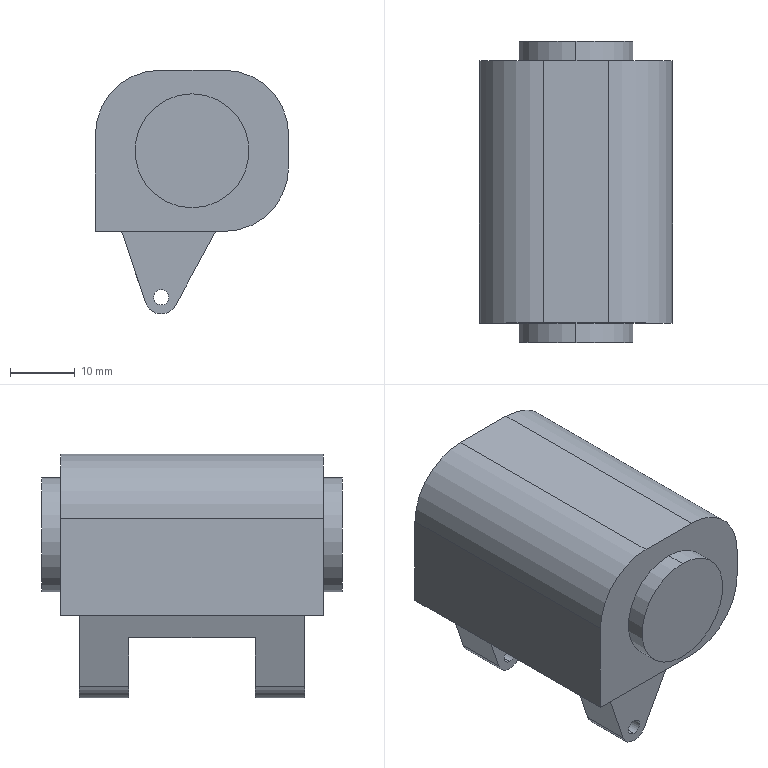Part | SolidWorks | features ICE 3, Cut 1, Extrusion 1, Fillet 1 | 1 solid | 28 faces | box 29.956 x 46.658 x 37.777 mm | volume 31870 mm3 | plane 15 | cylinder 13 | commonest cylinder face diameters 2.359 x4 17.683 x4 20 x3 5.115 x2
STEP:
#1=CARTESIAN_POINT('',(-25.009,23.329,21.342));
#2=VERTEX_POINT('',#1);
#3=CARTESIAN_POINT('',(-25.009,23.329,3.658));
#4=VERTEX_POINT('',#3);
#5=CARTESIAN_POINT('',(-25.009,23.329,12.5));
#6=DIRECTION('',(0.,1.,0.));
#7=DIRECTION('',(0.,0.,1.));
#8=AXIS2_PLACEMENT_3D('',#5,#6,#7);
#9=CIRCLE('',#8,8.842);
#10=EDGE_CURVE('',#2,#4,#9,.T.);
#11=ORIENTED_EDGE('',*,*,#10,.F.);
#12=CARTESIAN_POINT('',(-25.009,20.329,21.342));
#13=VERTEX_POINT('',#12);
#14=CARTESIAN_POINT('',(-25.009,23.329,21.342));
#15=DIRECTION('',(0.,-1.,0.));
#16=VECTOR('',#15,1000.);
#17=LINE('',#14,#16);
#18=EDGE_CURVE('',#2,#13,#17,.T.);
#19=ORIENTED_EDGE('',*,*,#18,.T.);
#20=CARTESIAN_POINT('',(-25.009,20.329,3.658));
#21=VERTEX_POINT('',#20);
#22=CARTESIAN_POINT('',(-25.009,20.329,12.5));
#23=DIRECTION('',(0.,1.,0.));
#24=DIRECTION('',(0.,0.,1.));
#25=AXIS2_PLACEMENT_3D('',#22,#23,#24);
#26=CIRCLE('',#25,8.842);
#27=EDGE_CURVE('',#13,#21,#26,.T.);
#28=ORIENTED_EDGE('',*,*,#27,.T.);
#29=CARTESIAN_POINT('',(-25.009,23.329,3.658));
#30=DIRECTION('',(0.,-1.,0.));
#31=VECTOR('',#30,1000.);
#32=LINE('',#29,#31);
#33=EDGE_CURVE('',#4,#21,#32,.T.);
#34=ORIENTED_EDGE('',*,*,#33,.F.);
#35=EDGE_LOOP('',(#11,#19,#28,#34));
#36=FACE_OUTER_BOUND('',#35,.T.);
#37=CARTESIAN_POINT('',(-25.009,23.329,12.5));
#38=DIRECTION('',(0.,-1.,0.));
#39=DIRECTION('',(0.,0.,-1.));
#40=AXIS2_PLACEMENT_3D('',#37,#38,#39);
#41=CYLINDRICAL_SURFACE('',#40,8.842);
#42=ADVANCED_FACE('',(#36),#41,.T.);
#43=CARTESIAN_POINT('',(-25.009,-23.329,3.658));
#44=VERTEX_POINT('',#43);
#45=CARTESIAN_POINT('',(-25.009,-23.329,21.342));
#46=VERTEX_POINT('',#45);
#47=CARTESIAN_POINT('',(-25.009,-23.329,12.5));
#48=DIRECTION('',(0.,-1.,0.));
#49=DIRECTION('',(0.,0.,-1.));
#50=AXIS2_PLACEMENT_3D('',#47,#48,#49);
#51=CIRCLE('',#50,8.842);
#52=EDGE_CURVE('',#44,#46,#51,.T.);
#53=ORIENTED_EDGE('',*,*,#52,.F.);
#54=CARTESIAN_POINT('',(-25.009,-20.329,3.658));
#55=VERTEX_POINT('',#54);
#56=CARTESIAN_POINT('',(-25.009,-23.329,3.658));
#57=DIRECTION('',(0.,1.,0.));
#58=VECTOR('',#57,1000.);
#59=LINE('',#56,#58);
#60=EDGE_CURVE('',#44,#55,#59,.T.);
#61=ORIENTED_EDGE('',*,*,#60,.T.);
#62=CARTESIAN_POINT('',(-25.009,-20.329,21.342));
#63=VERTEX_POINT('',#62);
#64=CARTESIAN_POINT('',(-25.009,-20.329,12.5));
#65=DIRECTION('',(0.,-1.,0.));
#66=DIRECTION('',(0.,0.,-1.));
#67=AXIS2_PLACEMENT_3D('',#64,#65,#66);
#68=CIRCLE('',#67,8.842);
#69=EDGE_CURVE('',#55,#63,#68,.T.);
#70=ORIENTED_EDGE('',*,*,#69,.T.);
#71=CARTESIAN_POINT('',(-25.009,-23.329,21.342));
#72=DIRECTION('',(0.,1.,0.));
#73=VECTOR('',#72,1000.);
#74=LINE('',#71,#73);
#75=EDGE_CURVE('',#46,#63,#74,.T.);
#76=ORIENTED_EDGE('',*,*,#75,.F.);
#77=EDGE_LOOP('',(#53,#61,#70,#76));
#78=FACE_OUTER_BOUND('',#77,.T.);
#79=CARTESIAN_POINT('',(-25.009,-23.329,12.5));
#80=DIRECTION('',(0.,1.,0.));
#81=DIRECTION('',(0.,0.,1.));
#82=AXIS2_PLACEMENT_3D('',#79,#80,#81);
#83=CYLINDRICAL_SURFACE('',#82,8.842);
#84=ADVANCED_FACE('',(#78),#83,.T.);
#85=CARTESIAN_POINT('',(-29.791,-17.5,-9.04));
#86=VERTEX_POINT('',#85);
#87=CARTESIAN_POINT('',(-29.791,-17.5,-11.399));
#88=VERTEX_POINT('',#87);
#89=CARTESIAN_POINT('',(-29.791,-17.5,-10.22));
#90=DIRECTION('',(0.,-1.,0.));
#91=DIRECTION('',(0.,0.,-1.));
#92=AXIS2_PLACEMENT_3D('',#89,#90,#91);
#93=CIRCLE('',#92,1.179);
#94=EDGE_CURVE('',#86,#88,#93,.T.);
#95=ORIENTED_EDGE('',*,*,#94,.T.);
#96=CARTESIAN_POINT('',(-29.791,-9.777,-11.399));
#97=VERTEX_POINT('',#96);
#98=CARTESIAN_POINT('',(-29.791,-17.5,-11.399));
#99=DIRECTION('',(0.,1.,0.));
#100=VECTOR('',#99,1000.);
#101=LINE('',#98,#100);
#102=EDGE_CURVE('',#88,#97,#101,.T.);
#103=ORIENTED_EDGE('',*,*,#102,.T.);
#104=CARTESIAN_POINT('',(-29.791,-9.777,-9.04));
#105=VERTEX_POINT('',#104);
#106=CARTESIAN_POINT('',(-29.791,-9.777,-10.22));
#107=DIRECTION('',(0.,-1.,0.));
#108=DIRECTION('',(0.,0.,-1.));
#109=AXIS2_PLACEMENT_3D('',#106,#107,#108);
#110=CIRCLE('',#109,1.179);
#111=EDGE_CURVE('',#105,#97,#110,.T.);
#112=ORIENTED_EDGE('',*,*,#111,.F.);
#113=CARTESIAN_POINT('',(-29.791,-17.5,-9.04));
#114=DIRECTION('',(0.,1.,0.));
#115=VECTOR('',#114,1000.);
#116=LINE('',#113,#115);
#117=EDGE_CURVE('',#86,#105,#116,.T.);
#118=ORIENTED_EDGE('',*,*,#117,.F.);
#119=EDGE_LOOP('',(#95,#103,#112,#118));
#120=FACE_OUTER_BOUND('',#119,.T.);
#121=CARTESIAN_POINT('',(-29.791,-17.5,-10.22));
#122=DIRECTION('',(0.,1.,0.));
#123=DIRECTION('',(0.,0.,1.));
#124=AXIS2_PLACEMENT_3D('',#121,#122,#123);
#125=CYLINDRICAL_SURFACE('',#124,1.179);
#126=ADVANCED_FACE('',(#120),#125,.F.);
#127=CARTESIAN_POINT('',(-29.791,9.777,-11.399));
#128=VERTEX_POINT('',#127);
#129=CARTESIAN_POINT('',(-29.791,9.777,-9.04));
#130=VERTEX_POINT('',#129);
#131=CARTESIAN_POINT('',(-29.791,9.777,-10.22));
#132=DIRECTION('',(0.,1.,0.));
#133=DIRECTION('',(0.,0.,1.));
#134=AXIS2_PLACEMENT_3D('',#131,#132,#133);
#135=CIRCLE('',#134,1.179);
#136=EDGE_CURVE('',#128,#130,#135,.T.);
#137=ORIENTED_EDGE('',*,*,#136,.F.);
#138=CARTESIAN_POINT('',(-29.791,17.5,-11.399));
#139=VERTEX_POINT('',#138);
#140=CARTESIAN_POINT('',(-29.791,-17.5,-11.399));
#141=DIRECTION('',(0.,1.,0.));
#142=VECTOR('',#141,1000.);
#143=LINE('',#140,#142);
#144=EDGE_CURVE('',#128,#139,#143,.T.);
#145=ORIENTED_EDGE('',*,*,#144,.T.);
#146=CARTESIAN_POINT('',(-29.791,17.5,-9.04));
#147=VERTEX_POINT('',#146);
#148=CARTESIAN_POINT('',(-29.791,17.5,-10.22));
#149=DIRECTION('',(0.,-1.,0.));
#150=DIRECTION('',(0.,0.,-1.));
#151=AXIS2_PLACEMENT_3D('',#148,#149,#150);
#152=CIRCLE('',#151,1.179);
#153=EDGE_CURVE('',#147,#139,#152,.T.);
#154=ORIENTED_EDGE('',*,*,#153,.F.);
#155=CARTESIAN_POINT('',(-29.791,-17.5,-9.04));
#156=DIRECTION('',(0.,1.,0.));
#157=VECTOR('',#156,1000.);
#158=LINE('',#155,#157);
#159=EDGE_CURVE('',#130,#147,#158,.T.);
#160=ORIENTED_EDGE('',*,*,#159,.F.);
#161=EDGE_LOOP('',(#137,#145,#154,#160));
#162=FACE_OUTER_BOUND('',#161,.T.);
#163=CARTESIAN_POINT('',(-29.791,-17.5,-10.22));
#164=DIRECTION('',(0.,1.,0.));
#165=DIRECTION('',(0.,0.,1.));
#166=AXIS2_PLACEMENT_3D('',#163,#164,#165);
#167=CYLINDRICAL_SURFACE('',#166,1.179);
#168=ADVANCED_FACE('',(#162),#167,.F.);
#169=CARTESIAN_POINT('',(-27.542,9.777,-11.438));
#170=VERTEX_POINT('',#169);
#171=CARTESIAN_POINT('',(-27.542,17.5,-11.438));
#172=VERTEX_POINT('',#171);
#173=CARTESIAN_POINT('',(-27.542,-17.5,-11.438));
#174=DIRECTION('',(0.,1.,0.));
#175=VECTOR('',#174,1000.);
#176=LINE('',#173,#175);
#177=EDGE_CURVE('',#170,#172,#176,.T.);
#178=ORIENTED_EDGE('',*,*,#177,.F.);
#179=CARTESIAN_POINT('',(-32.216,9.777,-11.033));
#180=VERTEX_POINT('',#179);
#181=CARTESIAN_POINT('',(-29.791,9.777,-10.22));
#182=DIRECTION('',(0.,1.,0.));
#183=DIRECTION('',(0.,0.,1.));
#184=AXIS2_PLACEMENT_3D('',#181,#182,#183);
#185=CIRCLE('',#184,2.558);
#186=EDGE_CURVE('',#170,#180,#185,.T.);
#187=ORIENTED_EDGE('',*,*,#186,.T.);
#188=CARTESIAN_POINT('',(-32.216,17.5,-11.033));
#189=VERTEX_POINT('',#188);
#190=CARTESIAN_POINT('',(-32.216,-17.5,-11.033));
#191=DIRECTION('',(0.,1.,0.));
#192=VECTOR('',#191,1000.);
#193=LINE('',#190,#192);
#194=EDGE_CURVE('',#180,#189,#193,.T.);
#195=ORIENTED_EDGE('',*,*,#194,.T.);
#196=CARTESIAN_POINT('',(-29.791,17.5,-10.22));
#197=DIRECTION('',(0.,-1.,0.));
#198=DIRECTION('',(0.,0.,-1.));
#199=AXIS2_PLACEMENT_3D('',#196,#197,#198);
#200=CIRCLE('',#199,2.558);
#201=EDGE_CURVE('',#189,#172,#200,.T.);
#202=ORIENTED_EDGE('',*,*,#201,.T.);
#203=EDGE_LOOP('',(#178,#187,#195,#202));
#204=FACE_OUTER_BOUND('',#203,.T.);
#205=CARTESIAN_POINT('',(-29.791,-17.5,-10.22));
#206=DIRECTION('',(0.,1.,0.));
#207=DIRECTION('',(0.,0.,1.));
#208=AXIS2_PLACEMENT_3D('',#205,#206,#207);
#209=CYLINDRICAL_SURFACE('',#208,2.558);
#210=ADVANCED_FACE('',(#204),#209,.T.);
#211=ORIENTED_EDGE('',*,*,#144,.F.);
#212=CARTESIAN_POINT('',(-29.791,9.777,-10.22));
#213=DIRECTION('',(0.,1.,0.));
#214=DIRECTION('',(0.,0.,1.));
#215=AXIS2_PLACEMENT_3D('',#212,#213,#214);
#216=CIRCLE('',#215,1.179);
#217=EDGE_CURVE('',#130,#128,#216,.T.);
#218=ORIENTED_EDGE('',*,*,#217,.F.);
#219=ORIENTED_EDGE('',*,*,#159,.T.);
#220=CARTESIAN_POINT('',(-29.791,17.5,-10.22));
#221=DIRECTION('',(0.,-1.,0.));
#222=DIRECTION('',(0.,0.,-1.));
#223=AXIS2_PLACEMENT_3D('',#220,#221,#222);
#224=CIRCLE('',#223,1.179);
#225=EDGE_CURVE('',#139,#147,#224,.T.);
#226=ORIENTED_EDGE('',*,*,#225,.F.);
#227=EDGE_LOOP('',(#211,#218,#219,#226));
#228=FACE_OUTER_BOUND('',#227,.T.);
#229=CARTESIAN_POINT('',(-29.791,-17.5,-10.22));
#230=DIRECTION('',(0.,1.,0.));
#231=DIRECTION('',(0.,0.,1.));
#232=AXIS2_PLACEMENT_3D('',#229,#230,#231);
#233=CYLINDRICAL_SURFACE('',#232,1.179);
#234=ADVANCED_FACE('',(#228),#233,.F.);
#235=CARTESIAN_POINT('',(-10.031,-20.329,15.));
#236=VERTEX_POINT('',#235);
#237=CARTESIAN_POINT('',(-10.031,-20.329,10.));
#238=VERTEX_POINT('',#237);
#239=CARTESIAN_POINT('',(-10.031,-20.329,25.));
#240=DIRECTION('',(0.,0.,-1.));
#241=VECTOR('',#240,1000.);
#242=LINE('',#239,#241);
#243=EDGE_CURVE('',#236,#238,#242,.T.);
#244=ORIENTED_EDGE('',*,*,#243,.T.);
#245=CARTESIAN_POINT('',(-10.031,20.329,10.));
#246=VERTEX_POINT('',#245);
#247=CARTESIAN_POINT('',(-10.031,20.329,10.));
#248=DIRECTION('',(0.,1.,0.));
#249=VECTOR('',#248,1000.);
#250=LINE('',#247,#249);
#251=EDGE_CURVE('',#238,#246,#250,.T.);
#252=ORIENTED_EDGE('',*,*,#251,.T.);
#253=CARTESIAN_POINT('',(-10.031,20.329,15.));
#254=VERTEX_POINT('',#253);
#255=CARTESIAN_POINT('',(-10.031,20.329,25.));
#256=DIRECTION('',(0.,0.,-1.));
#257=VECTOR('',#256,1000.);
#258=LINE('',#255,#257);
#259=EDGE_CURVE('',#254,#246,#258,.T.);
#260=ORIENTED_EDGE('',*,*,#259,.F.);
#261=CARTESIAN_POINT('',(-10.031,-20.329,15.));
#262=DIRECTION('',(0.,-1.,0.));
#263=VECTOR('',#262,1000.);
#264=LINE('',#261,#263);
#265=EDGE_CURVE('',#254,#236,#264,.T.);
#266=ORIENTED_EDGE('',*,*,#265,.T.);
#267=EDGE_LOOP('',(#244,#252,#260,#266));
#268=FACE_OUTER_BOUND('',#267,.T.);
#269=CARTESIAN_POINT('',(-10.031,20.329,25.));
#270=DIRECTION('',(-1.,0.,0.));
#271=DIRECTION('',(0.,0.,1.));
#272=AXIS2_PLACEMENT_3D('',#269,#270,#271);
#273=PLANE('',#272);
#274=ADVANCED_FACE('',(#268),#273,.F.);
#275=CARTESIAN_POINT('',(-25.009,20.329,12.5));
#276=DIRECTION('',(0.,1.,0.));
#277=DIRECTION('',(0.,0.,1.));
#278=AXIS2_PLACEMENT_3D('',#275,#276,#277);
#279=CIRCLE('',#278,8.842);
#280=EDGE_CURVE('',#21,#13,#279,.T.);
#281=ORIENTED_EDGE('',*,*,#280,.F.);
#282=ORIENTED_EDGE('',*,*,#27,.F.);
#283=EDGE_LOOP('',(#281,#282));
#284=FACE_BOUND('',#283,.T.);
#285=CARTESIAN_POINT('',(-39.987,20.329,15.));
#286=VERTEX_POINT('',#285);
#287=CARTESIAN_POINT('',(-39.987,20.329,0.));
#288=VERTEX_POINT('',#287);
#289=CARTESIAN_POINT('',(-39.987,20.329,25.));
#290=DIRECTION('',(0.,0.,-1.));
#291=VECTOR('',#290,1000.);
#292=LINE('',#289,#291);
#293=EDGE_CURVE('',#286,#288,#292,.T.);
#294=ORIENTED_EDGE('',*,*,#293,.F.);
#295=CARTESIAN_POINT('',(-29.987,20.329,25.));
#296=VERTEX_POINT('',#295);
#297=CARTESIAN_POINT('',(-29.987,20.329,15.));
#298=DIRECTION('',(0.,1.,0.));
#299=DIRECTION('',(0.,0.,-1.));
#300=AXIS2_PLACEMENT_3D('',#297,#298,#299);
#301=CIRCLE('',#300,10.);
#302=EDGE_CURVE('',#286,#296,#301,.T.);
#303=ORIENTED_EDGE('',*,*,#302,.T.);
#304=CARTESIAN_POINT('',(-20.031,20.329,25.));
#305=VERTEX_POINT('',#304);
#306=CARTESIAN_POINT('',(-39.987,20.329,25.));
#307=DIRECTION('',(-1.,0.,0.));
#308=VECTOR('',#307,1000.);
#309=LINE('',#306,#308);
#310=EDGE_CURVE('',#305,#296,#309,.T.);
#311=ORIENTED_EDGE('',*,*,#310,.F.);
#312=CARTESIAN_POINT('',(-20.031,20.329,15.));
#313=DIRECTION('',(0.,1.,0.));
#314=DIRECTION('',(0.,0.,-1.));
#315=AXIS2_PLACEMENT_3D('',#312,#313,#314);
#316=CIRCLE('',#315,10.);
#317=EDGE_CURVE('',#305,#254,#316,.T.);
#318=ORIENTED_EDGE('',*,*,#317,.T.);
#319=ORIENTED_EDGE('',*,*,#259,.T.);
#320=CARTESIAN_POINT('',(-20.031,20.329,0.));
#321=VERTEX_POINT('',#320);
#322=CARTESIAN_POINT('',(-20.031,20.329,10.));
#323=DIRECTION('',(0.,1.,0.));
#324=DIRECTION('',(0.,0.,-1.));
#325=AXIS2_PLACEMENT_3D('',#322,#323,#324);
#326=CIRCLE('',#325,10.);
#327=EDGE_CURVE('',#246,#321,#326,.T.);
#328=ORIENTED_EDGE('',*,*,#327,.T.);
#329=CARTESIAN_POINT('',(-39.987,20.329,0.));
#330=DIRECTION('',(-1.,0.,0.));
#331=VECTOR('',#330,1000.);
#332=LINE('',#329,#331);
#333=EDGE_CURVE('',#321,#288,#332,.T.);
#334=ORIENTED_EDGE('',*,*,#333,.T.);
#335=EDGE_LOOP('',(#294,#303,#311,#318,#319,#328,#334));
#336=FACE_OUTER_BOUND('',#335,.T.);
#337=CARTESIAN_POINT('',(-39.987,20.329,25.));
#338=DIRECTION('',(0.,-1.,0.));
#339=DIRECTION('',(0.,0.,-1.));
#340=AXIS2_PLACEMENT_3D('',#337,#338,#339);
#341=PLANE('',#340);
#342=ADVANCED_FACE('',(#284,#336),#341,.F.);
#343=CARTESIAN_POINT('',(-39.987,-20.329,15.));
#344=VERTEX_POINT('',#343);
#345=CARTESIAN_POINT('',(-39.987,-20.329,0.));
#346=VERTEX_POINT('',#345);
#347=CARTESIAN_POINT('',(-39.987,-20.329,25.));
#348=DIRECTION('',(0.,0.,-1.));
#349=VECTOR('',#348,1000.);
#350=LINE('',#347,#349);
#351=EDGE_CURVE('',#344,#346,#350,.T.);
#352=ORIENTED_EDGE('',*,*,#351,.F.);
#353=CARTESIAN_POINT('',(-39.987,20.329,15.));
#354=DIRECTION('',(0.,1.,0.));
#355=VECTOR('',#354,1000.);
#356=LINE('',#353,#355);
#357=EDGE_CURVE('',#344,#286,#356,.T.);
#358=ORIENTED_EDGE('',*,*,#357,.T.);
#359=ORIENTED_EDGE('',*,*,#293,.T.);
#360=CARTESIAN_POINT('',(-39.987,20.329,0.));
#361=DIRECTION('',(0.,-1.,0.));
#362=VECTOR('',#361,1000.);
#363=LINE('',#360,#362);
#364=EDGE_CURVE('',#288,#346,#363,.T.);
#365=ORIENTED_EDGE('',*,*,#364,.T.);
#366=EDGE_LOOP('',(#352,#358,#359,#365));
#367=FACE_OUTER_BOUND('',#366,.T.);
#368=CARTESIAN_POINT('',(-39.987,20.329,25.));
#369=DIRECTION('',(1.,0.,0.));
#370=DIRECTION('',(0.,0.,-1.));
#371=AXIS2_PLACEMENT_3D('',#368,#369,#370);
#372=PLANE('',#371);
#373=ADVANCED_FACE('',(#367),#372,.F.);
#374=CARTESIAN_POINT('',(-25.009,-20.329,12.5));
#375=DIRECTION('',(0.,-1.,0.));
#376=DIRECTION('',(0.,0.,-1.));
#377=AXIS2_PLACEMENT_3D('',#374,#375,#376);
#378=CIRCLE('',#377,8.842);
#379=EDGE_CURVE('',#63,#55,#378,.T.);
#380=ORIENTED_EDGE('',*,*,#379,.F.);
#381=ORIENTED_EDGE('',*,*,#69,.F.);
#382=EDGE_LOOP('',(#380,#381));
#383=FACE_BOUND('',#382,.T.);
#384=CARTESIAN_POINT('',(-29.987,-20.329,25.));
#385=VERTEX_POINT('',#384);
#386=CARTESIAN_POINT('',(-20.031,-20.329,25.));
#387=VERTEX_POINT('',#386);
#388=CARTESIAN_POINT('',(-39.987,-20.329,25.));
#389=DIRECTION('',(1.,0.,0.));
#390=VECTOR('',#389,1000.);
#391=LINE('',#388,#390);
#392=EDGE_CURVE('',#385,#387,#391,.T.);
#393=ORIENTED_EDGE('',*,*,#392,.F.);
#394=CARTESIAN_POINT('',(-29.987,-20.329,15.));
#395=DIRECTION('',(0.,-1.,0.));
#396=DIRECTION('',(0.,0.,1.));
#397=AXIS2_PLACEMENT_3D('',#394,#395,#396);
#398=CIRCLE('',#397,10.);
#399=EDGE_CURVE('',#385,#344,#398,.T.);
#400=ORIENTED_EDGE('',*,*,#399,.T.);
#401=ORIENTED_EDGE('',*,*,#351,.T.);
#402=CARTESIAN_POINT('',(-20.031,-20.329,0.));
#403=VERTEX_POINT('',#402);
#404=CARTESIAN_POINT('',(-39.987,-20.329,0.));
#405=DIRECTION('',(1.,0.,0.));
#406=VECTOR('',#405,1000.);
#407=LINE('',#404,#406);
#408=EDGE_CURVE('',#346,#403,#407,.T.);
#409=ORIENTED_EDGE('',*,*,#408,.T.);
#410=CARTESIAN_POINT('',(-20.031,-20.329,10.));
#411=DIRECTION('',(0.,-1.,0.));
#412=DIRECTION('',(0.,0.,1.));
#413=AXIS2_PLACEMENT_3D('',#410,#411,#412);
#414=CIRCLE('',#413,10.);
#415=EDGE_CURVE('',#403,#238,#414,.T.);
#416=ORIENTED_EDGE('',*,*,#415,.T.);
#417=ORIENTED_EDGE('',*,*,#243,.F.);
#418=CARTESIAN_POINT('',(-20.031,-20.329,15.));
#419=DIRECTION('',(0.,-1.,0.));
#420=DIRECTION('',(0.,0.,1.));
#421=AXIS2_PLACEMENT_3D('',#418,#419,#420);
#422=CIRCLE('',#421,10.);
#423=EDGE_CURVE('',#236,#387,#422,.T.);
#424=ORIENTED_EDGE('',*,*,#423,.T.);
#425=EDGE_LOOP('',(#393,#400,#401,#409,#416,#417,#424));
#426=FACE_OUTER_BOUND('',#425,.T.);
#427=CARTESIAN_POINT('',(-39.987,-20.329,25.));
#428=DIRECTION('',(0.,1.,0.));
#429=DIRECTION('',(0.,0.,1.));
#430=AXIS2_PLACEMENT_3D('',#427,#428,#429);
#431=PLANE('',#430);
#432=ADVANCED_FACE('',(#383,#426),#431,.F.);
#433=ORIENTED_EDGE('',*,*,#310,.T.);
#434=CARTESIAN_POINT('',(-29.987,-20.329,25.));
#435=DIRECTION('',(0.,-1.,0.));
#436=VECTOR('',#435,1000.);
#437=LINE('',#434,#436);
#438=EDGE_CURVE('',#296,#385,#437,.T.);
#439=ORIENTED_EDGE('',*,*,#438,.T.);
#440=ORIENTED_EDGE('',*,*,#392,.T.);
#441=CARTESIAN_POINT('',(-20.031,20.329,25.));
#442=DIRECTION('',(0.,1.,0.));
#443=VECTOR('',#442,1000.);
#444=LINE('',#441,#443);
#445=EDGE_CURVE('',#387,#305,#444,.T.);
#446=ORIENTED_EDGE('',*,*,#445,.T.);
#447=EDGE_LOOP('',(#433,#439,#440,#446));
#448=FACE_OUTER_BOUND('',#447,.T.);
#449=CARTESIAN_POINT('',(0.,0.,25.));
#450=DIRECTION('',(0.,0.,1.));
#451=DIRECTION('',(1.,0.,0.));
#452=AXIS2_PLACEMENT_3D('',#449,#450,#451);
#453=PLANE('',#452);
#454=ADVANCED_FACE('',(#448),#453,.T.);
#455=CARTESIAN_POINT('',(-21.346,-17.5,0.));
#456=VERTEX_POINT('',#455);
#457=CARTESIAN_POINT('',(-21.346,17.5,0.));
#458=VERTEX_POINT('',#457);
#459=CARTESIAN_POINT('',(-21.346,-17.5,0.));
#460=DIRECTION('',(0.,1.,0.));
#461=VECTOR('',#460,1000.);
#462=LINE('',#459,#461);
#463=EDGE_CURVE('',#456,#458,#462,.T.);
#464=ORIENTED_EDGE('',*,*,#463,.T.);
#465=CARTESIAN_POINT('',(-35.914,17.5,0.));
#466=VERTEX_POINT('',#465);
#467=CARTESIAN_POINT('',(-21.346,17.5,0.));
#468=DIRECTION('',(-1.,0.,0.));
#469=VECTOR('',#468,1000.);
#470=LINE('',#467,#469);
#471=EDGE_CURVE('',#458,#466,#470,.T.);
#472=ORIENTED_EDGE('',*,*,#471,.T.);
#473=CARTESIAN_POINT('',(-35.914,-17.5,0.));
#474=VERTEX_POINT('',#473);
#475=CARTESIAN_POINT('',(-35.914,-17.5,0.));
#476=DIRECTION('',(0.,1.,0.));
#477=VECTOR('',#476,1000.);
#478=LINE('',#475,#477);
#479=EDGE_CURVE('',#474,#466,#478,.T.);
#480=ORIENTED_EDGE('',*,*,#479,.F.);
#481=CARTESIAN_POINT('',(-21.346,-17.5,0.));
#482=DIRECTION('',(-1.,0.,0.));
#483=VECTOR('',#482,1000.);
#484=LINE('',#481,#483);
#485=EDGE_CURVE('',#456,#474,#484,.T.);
#486=ORIENTED_EDGE('',*,*,#485,.F.);
#487=EDGE_LOOP('',(#464,#472,#480,#486));
#488=FACE_BOUND('',#487,.T.);
#489=ORIENTED_EDGE('',*,*,#333,.F.);
#490=CARTESIAN_POINT('',(-20.031,0.,0.));
#491=DIRECTION('',(0.,-1.,0.));
#492=VECTOR('',#491,1000.);
#493=LINE('',#490,#492);
#494=EDGE_CURVE('',#321,#403,#493,.T.);
#495=ORIENTED_EDGE('',*,*,#494,.T.);
#496=ORIENTED_EDGE('',*,*,#408,.F.);
#497=ORIENTED_EDGE('',*,*,#364,.F.);
#498=EDGE_LOOP('',(#489,#495,#496,#497));
#499=FACE_OUTER_BOUND('',#498,.T.);
#500=CARTESIAN_POINT('',(0.,0.,0.));
#501=DIRECTION('',(0.,0.,1.));
#502=DIRECTION('',(1.,0.,0.));
#503=AXIS2_PLACEMENT_3D('',#500,#501,#502);
#504=PLANE('',#503);
#505=ADVANCED_FACE('',(#488,#499),#504,.F.);
#506=CARTESIAN_POINT('',(-32.216,-17.5,-11.033));
#507=VERTEX_POINT('',#506);
#508=CARTESIAN_POINT('',(-27.542,-17.5,-11.438));
#509=VERTEX_POINT('',#508);
#510=CARTESIAN_POINT('',(-29.791,-17.5,-10.22));
#511=DIRECTION('',(0.,-1.,0.));
#512=DIRECTION('',(0.,0.,-1.));
#513=AXIS2_PLACEMENT_3D('',#510,#511,#512);
#514=CIRCLE('',#513,2.558);
#515=EDGE_CURVE('',#507,#509,#514,.T.);
#516=ORIENTED_EDGE('',*,*,#515,.T.);
#517=CARTESIAN_POINT('',(-27.542,-17.5,-11.438));
#518=DIRECTION('',(0.4763,0.,0.8793));
#519=VECTOR('',#518,1000.);
#520=LINE('',#517,#519);
#521=EDGE_CURVE('',#509,#456,#520,.T.);
#522=ORIENTED_EDGE('',*,*,#521,.T.);
#523=ORIENTED_EDGE('',*,*,#485,.T.);
#524=CARTESIAN_POINT('',(-32.216,-17.5,-11.033));
#525=DIRECTION('',(0.3178,0.,-0.9482));
#526=VECTOR('',#525,1000.);
#527=LINE('',#524,#526);
#528=EDGE_CURVE('',#474,#507,#527,.T.);
#529=ORIENTED_EDGE('',*,*,#528,.T.);
#530=EDGE_LOOP('',(#516,#522,#523,#529));
#531=FACE_OUTER_BOUND('',#530,.T.);
#532=ORIENTED_EDGE('',*,*,#94,.F.);
#533=CARTESIAN_POINT('',(-29.791,-17.5,-10.22));
#534=DIRECTION('',(0.,-1.,0.));
#535=DIRECTION('',(0.,0.,-1.));
#536=AXIS2_PLACEMENT_3D('',#533,#534,#535);
#537=CIRCLE('',#536,1.179);
#538=EDGE_CURVE('',#88,#86,#537,.T.);
#539=ORIENTED_EDGE('',*,*,#538,.F.);
#540=EDGE_LOOP('',(#532,#539));
#541=FACE_BOUND('',#540,.T.);
#542=CARTESIAN_POINT('',(-29.791,-17.5,-10.22));
#543=DIRECTION('',(0.,-1.,0.));
#544=DIRECTION('',(0.,0.,-1.));
#545=AXIS2_PLACEMENT_3D('',#542,#543,#544);
#546=PLANE('',#545);
#547=ADVANCED_FACE('',(#531,#541),#546,.T.);
#548=ORIENTED_EDGE('',*,*,#201,.F.);
#549=CARTESIAN_POINT('',(-32.216,17.5,-11.033));
#550=DIRECTION('',(0.3178,0.,-0.9482));
#551=VECTOR('',#550,1000.);
#552=LINE('',#549,#551);
#553=EDGE_CURVE('',#466,#189,#552,.T.);
#554=ORIENTED_EDGE('',*,*,#553,.F.);
#555=ORIENTED_EDGE('',*,*,#471,.F.);
#556=CARTESIAN_POINT('',(-27.542,17.5,-11.438));
#557=DIRECTION('',(0.4763,0.,0.8793));
#558=VECTOR('',#557,1000.);
#559=LINE('',#556,#558);
#560=EDGE_CURVE('',#172,#458,#559,.T.);
#561=ORIENTED_EDGE('',*,*,#560,.F.);
#562=EDGE_LOOP('',(#548,#554,#555,#561));
#563=FACE_OUTER_BOUND('',#562,.T.);
#564=ORIENTED_EDGE('',*,*,#153,.T.);
#565=ORIENTED_EDGE('',*,*,#225,.T.);
#566=EDGE_LOOP('',(#564,#565));
#567=FACE_BOUND('',#566,.T.);
#568=CARTESIAN_POINT('',(-29.791,17.5,-10.22));
#569=DIRECTION('',(0.,-1.,0.));
#570=DIRECTION('',(0.,0.,-1.));
#571=AXIS2_PLACEMENT_3D('',#568,#569,#570);
#572=PLANE('',#571);
#573=ADVANCED_FACE('',(#563,#567),#572,.F.);
#574=CARTESIAN_POINT('',(-32.216,-9.777,-11.033));
#575=VERTEX_POINT('',#574);
#576=CARTESIAN_POINT('',(-32.216,-17.5,-11.033));
#577=DIRECTION('',(0.,1.,0.));
#578=VECTOR('',#577,1000.);
#579=LINE('',#576,#578);
#580=EDGE_CURVE('',#507,#575,#579,.T.);
#581=ORIENTED_EDGE('',*,*,#580,.T.);
#582=CARTESIAN_POINT('',(-27.542,-9.777,-11.438));
#583=VERTEX_POINT('',#582);
#584=CARTESIAN_POINT('',(-29.791,-9.777,-10.22));
#585=DIRECTION('',(0.,-1.,0.));
#586=DIRECTION('',(0.,0.,-1.));
#587=AXIS2_PLACEMENT_3D('',#584,#585,#586);
#588=CIRCLE('',#587,2.558);
#589=EDGE_CURVE('',#575,#583,#588,.T.);
#590=ORIENTED_EDGE('',*,*,#589,.T.);
#591=CARTESIAN_POINT('',(-27.542,-17.5,-11.438));
#592=DIRECTION('',(0.,1.,0.));
#593=VECTOR('',#592,1000.);
#594=LINE('',#591,#593);
#595=EDGE_CURVE('',#509,#583,#594,.T.);
#596=ORIENTED_EDGE('',*,*,#595,.F.);
#597=ORIENTED_EDGE('',*,*,#515,.F.);
#598=EDGE_LOOP('',(#581,#590,#596,#597));
#599=FACE_OUTER_BOUND('',#598,.T.);
#600=CARTESIAN_POINT('',(-29.791,-17.5,-10.22));
#601=DIRECTION('',(0.,1.,0.));
#602=DIRECTION('',(0.,0.,1.));
#603=AXIS2_PLACEMENT_3D('',#600,#601,#602);
#604=CYLINDRICAL_SURFACE('',#603,2.558);
#605=ADVANCED_FACE('',(#599),#604,.T.);
#606=CARTESIAN_POINT('',(-23.21,-9.777,-3.441));
#607=VERTEX_POINT('',#606);
#608=CARTESIAN_POINT('',(-23.21,9.777,-3.441));
#609=VERTEX_POINT('',#608);
#610=CARTESIAN_POINT('',(-23.21,-17.5,-3.441));
#611=DIRECTION('',(0.,1.,0.));
#612=VECTOR('',#611,1000.);
#613=LINE('',#610,#612);
#614=EDGE_CURVE('',#607,#609,#613,.T.);
#615=ORIENTED_EDGE('',*,*,#614,.T.);
#616=CARTESIAN_POINT('',(-27.542,9.777,-11.438));
#617=DIRECTION('',(-0.4763,0.,-0.8793));
#618=VECTOR('',#617,1000.);
#619=LINE('',#616,#618);
#620=EDGE_CURVE('',#609,#170,#619,.T.);
#621=ORIENTED_EDGE('',*,*,#620,.T.);
#622=ORIENTED_EDGE('',*,*,#177,.T.);
#623=ORIENTED_EDGE('',*,*,#560,.T.);
#624=ORIENTED_EDGE('',*,*,#463,.F.);
#625=ORIENTED_EDGE('',*,*,#521,.F.);
#626=ORIENTED_EDGE('',*,*,#595,.T.);
#627=CARTESIAN_POINT('',(-27.542,-9.777,-11.438));
#628=DIRECTION('',(0.4763,0.,0.8793));
#629=VECTOR('',#628,1000.);
#630=LINE('',#627,#629);
#631=EDGE_CURVE('',#583,#607,#630,.T.);
#632=ORIENTED_EDGE('',*,*,#631,.T.);
#633=EDGE_LOOP('',(#615,#621,#622,#623,#624,#625,#626,#632));
#634=FACE_OUTER_BOUND('',#633,.T.);
#635=CARTESIAN_POINT('',(-27.542,-17.5,-11.438));
#636=DIRECTION('',(-0.8793,0.,0.4763));
#637=DIRECTION('',(0.4763,0.,0.8793));
#638=AXIS2_PLACEMENT_3D('',#635,#636,#637);
#639=PLANE('',#638);
#640=ADVANCED_FACE('',(#634),#639,.F.);
#641=ORIENTED_EDGE('',*,*,#194,.F.);
#642=CARTESIAN_POINT('',(-34.761,9.777,-3.441));
#643=VERTEX_POINT('',#642);
#644=CARTESIAN_POINT('',(-32.216,9.777,-11.033));
#645=DIRECTION('',(-0.3178,0.,0.9482));
#646=VECTOR('',#645,1000.);
#647=LINE('',#644,#646);
#648=EDGE_CURVE('',#180,#643,#647,.T.);
#649=ORIENTED_EDGE('',*,*,#648,.T.);
#650=CARTESIAN_POINT('',(-34.761,-9.777,-3.441));
#651=VERTEX_POINT('',#650);
#652=CARTESIAN_POINT('',(-34.761,-17.5,-3.441));
#653=DIRECTION('',(0.,-1.,0.));
#654=VECTOR('',#653,1000.);
#655=LINE('',#652,#654);
#656=EDGE_CURVE('',#643,#651,#655,.T.);
#657=ORIENTED_EDGE('',*,*,#656,.T.);
#658=CARTESIAN_POINT('',(-32.216,-9.777,-11.033));
#659=DIRECTION('',(0.3178,0.,-0.9482));
#660=VECTOR('',#659,1000.);
#661=LINE('',#658,#660);
#662=EDGE_CURVE('',#651,#575,#661,.T.);
#663=ORIENTED_EDGE('',*,*,#662,.T.);
#664=ORIENTED_EDGE('',*,*,#580,.F.);
#665=ORIENTED_EDGE('',*,*,#528,.F.);
#666=ORIENTED_EDGE('',*,*,#479,.T.);
#667=ORIENTED_EDGE('',*,*,#553,.T.);
#668=EDGE_LOOP('',(#641,#649,#657,#663,#664,#665,#666,#667));
#669=FACE_OUTER_BOUND('',#668,.T.);
#670=CARTESIAN_POINT('',(-32.216,-17.5,-11.033));
#671=DIRECTION('',(0.9482,0.,0.3178));
#672=DIRECTION('',(0.3178,0.,-0.9482));
#673=AXIS2_PLACEMENT_3D('',#670,#671,#672);
#674=PLANE('',#673);
#675=ADVANCED_FACE('',(#669),#674,.F.);
#676=ORIENTED_EDGE('',*,*,#102,.F.);
#677=ORIENTED_EDGE('',*,*,#538,.T.);
#678=ORIENTED_EDGE('',*,*,#117,.T.);
#679=CARTESIAN_POINT('',(-29.791,-9.777,-10.22));
#680=DIRECTION('',(0.,-1.,0.));
#681=DIRECTION('',(0.,0.,-1.));
#682=AXIS2_PLACEMENT_3D('',#679,#680,#681);
#683=CIRCLE('',#682,1.179);
#684=EDGE_CURVE('',#97,#105,#683,.T.);
#685=ORIENTED_EDGE('',*,*,#684,.F.);
#686=EDGE_LOOP('',(#676,#677,#678,#685));
#687=FACE_OUTER_BOUND('',#686,.T.);
#688=CARTESIAN_POINT('',(-29.791,-17.5,-10.22));
#689=DIRECTION('',(0.,1.,0.));
#690=DIRECTION('',(0.,0.,1.));
#691=AXIS2_PLACEMENT_3D('',#688,#689,#690);
#692=CYLINDRICAL_SURFACE('',#691,1.179);
#693=ADVANCED_FACE('',(#687),#692,.F.);
#694=ORIENTED_EDGE('',*,*,#302,.F.);
#695=ORIENTED_EDGE('',*,*,#357,.F.);
#696=ORIENTED_EDGE('',*,*,#399,.F.);
#697=ORIENTED_EDGE('',*,*,#438,.F.);
#698=EDGE_LOOP('',(#694,#695,#696,#697));
#699=FACE_OUTER_BOUND('',#698,.T.);
#700=CARTESIAN_POINT('',(-29.987,0.,15.));
#701=DIRECTION('',(0.,1.,0.));
#702=DIRECTION('',(0.,0.,1.));
#703=AXIS2_PLACEMENT_3D('',#700,#701,#702);
#704=CYLINDRICAL_SURFACE('',#703,10.);
#705=ADVANCED_FACE('',(#699),#704,.T.);
#706=ORIENTED_EDGE('',*,*,#415,.F.);
#707=ORIENTED_EDGE('',*,*,#494,.F.);
#708=ORIENTED_EDGE('',*,*,#327,.F.);
#709=ORIENTED_EDGE('',*,*,#251,.F.);
#710=EDGE_LOOP('',(#706,#707,#708,#709));
#711=FACE_OUTER_BOUND('',#710,.T.);
#712=CARTESIAN_POINT('',(-20.031,20.329,10.));
#713=DIRECTION('',(0.,1.,0.));
#714=DIRECTION('',(0.,0.,1.));
#715=AXIS2_PLACEMENT_3D('',#712,#713,#714);
#716=CYLINDRICAL_SURFACE('',#715,10.);
#717=ADVANCED_FACE('',(#711),#716,.T.);
#718=ORIENTED_EDGE('',*,*,#423,.F.);
#719=ORIENTED_EDGE('',*,*,#265,.F.);
#720=ORIENTED_EDGE('',*,*,#317,.F.);
#721=ORIENTED_EDGE('',*,*,#445,.F.);
#722=EDGE_LOOP('',(#718,#719,#720,#721));
#723=FACE_OUTER_BOUND('',#722,.T.);
#724=CARTESIAN_POINT('',(-20.031,0.,15.));
#725=DIRECTION('',(0.,-1.,0.));
#726=DIRECTION('',(0.,0.,-1.));
#727=AXIS2_PLACEMENT_3D('',#724,#725,#726);
#728=CYLINDRICAL_SURFACE('',#727,10.);
#729=ADVANCED_FACE('',(#723),#728,.T.);
#730=ORIENTED_EDGE('',*,*,#60,.F.);
#731=CARTESIAN_POINT('',(-25.009,-23.329,12.5));
#732=DIRECTION('',(0.,-1.,0.));
#733=DIRECTION('',(0.,0.,-1.));
#734=AXIS2_PLACEMENT_3D('',#731,#732,#733);
#735=CIRCLE('',#734,8.842);
#736=EDGE_CURVE('',#46,#44,#735,.T.);
#737=ORIENTED_EDGE('',*,*,#736,.F.);
#738=ORIENTED_EDGE('',*,*,#75,.T.);
#739=ORIENTED_EDGE('',*,*,#379,.T.);
#740=EDGE_LOOP('',(#730,#737,#738,#739));
#741=FACE_OUTER_BOUND('',#740,.T.);
#742=CARTESIAN_POINT('',(-25.009,-23.329,12.5));
#743=DIRECTION('',(0.,1.,0.));
#744=DIRECTION('',(0.,0.,1.));
#745=AXIS2_PLACEMENT_3D('',#742,#743,#744);
#746=CYLINDRICAL_SURFACE('',#745,8.842);
#747=ADVANCED_FACE('',(#741),#746,.T.);
#748=ORIENTED_EDGE('',*,*,#736,.T.);
#749=ORIENTED_EDGE('',*,*,#52,.T.);
#750=EDGE_LOOP('',(#748,#749));
#751=FACE_OUTER_BOUND('',#750,.T.);
#752=CARTESIAN_POINT('',(-25.009,-23.329,12.5));
#753=DIRECTION('',(0.,-1.,0.));
#754=DIRECTION('',(0.,0.,-1.));
#755=AXIS2_PLACEMENT_3D('',#752,#753,#754);
#756=PLANE('',#755);
#757=ADVANCED_FACE('',(#751),#756,.T.);
#758=ORIENTED_EDGE('',*,*,#18,.F.);
#759=CARTESIAN_POINT('',(-25.009,23.329,12.5));
#760=DIRECTION('',(0.,1.,0.));
#761=DIRECTION('',(0.,0.,1.));
#762=AXIS2_PLACEMENT_3D('',#759,#760,#761);
#763=CIRCLE('',#762,8.842);
#764=EDGE_CURVE('',#4,#2,#763,.T.);
#765=ORIENTED_EDGE('',*,*,#764,.F.);
#766=ORIENTED_EDGE('',*,*,#33,.T.);
#767=ORIENTED_EDGE('',*,*,#280,.T.);
#768=EDGE_LOOP('',(#758,#765,#766,#767));
#769=FACE_OUTER_BOUND('',#768,.T.);
#770=CARTESIAN_POINT('',(-25.009,23.329,12.5));
#771=DIRECTION('',(0.,-1.,0.));
#772=DIRECTION('',(0.,0.,-1.));
#773=AXIS2_PLACEMENT_3D('',#770,#771,#772);
#774=CYLINDRICAL_SURFACE('',#773,8.842);
#775=ADVANCED_FACE('',(#769),#774,.T.);
#776=ORIENTED_EDGE('',*,*,#764,.T.);
#777=ORIENTED_EDGE('',*,*,#10,.T.);
#778=EDGE_LOOP('',(#776,#777));
#779=FACE_OUTER_BOUND('',#778,.T.);
#780=CARTESIAN_POINT('',(-25.009,23.329,12.5));
#781=DIRECTION('',(0.,1.,0.));
#782=DIRECTION('',(0.,0.,1.));
#783=AXIS2_PLACEMENT_3D('',#780,#781,#782);
#784=PLANE('',#783);
#785=ADVANCED_FACE('',(#779),#784,.T.);
#786=CARTESIAN_POINT('',(-11.987,-9.777,-3.441));
#787=DIRECTION('',(-1.,0.,0.));
#788=VECTOR('',#787,1000.);
#789=LINE('',#786,#788);
#790=EDGE_CURVE('',#607,#651,#789,.T.);
#791=ORIENTED_EDGE('',*,*,#790,.T.);
#792=ORIENTED_EDGE('',*,*,#656,.F.);
#793=CARTESIAN_POINT('',(-11.987,9.777,-3.441));
#794=DIRECTION('',(-1.,0.,0.));
#795=VECTOR('',#794,1000.);
#796=LINE('',#793,#795);
#797=EDGE_CURVE('',#609,#643,#796,.T.);
#798=ORIENTED_EDGE('',*,*,#797,.F.);
#799=ORIENTED_EDGE('',*,*,#614,.F.);
#800=EDGE_LOOP('',(#791,#792,#798,#799));
#801=FACE_OUTER_BOUND('',#800,.T.);
#802=CARTESIAN_POINT('',(-11.987,9.777,-3.441));
#803=DIRECTION('',(0.,0.,1.));
#804=DIRECTION('',(1.,0.,0.));
#805=AXIS2_PLACEMENT_3D('',#802,#803,#804);
#806=PLANE('',#805);
#807=ADVANCED_FACE('',(#801),#806,.F.);
#808=ORIENTED_EDGE('',*,*,#217,.T.);
#809=ORIENTED_EDGE('',*,*,#136,.T.);
#810=EDGE_LOOP('',(#808,#809));
#811=FACE_BOUND('',#810,.T.);
#812=ORIENTED_EDGE('',*,*,#797,.T.);
#813=ORIENTED_EDGE('',*,*,#648,.F.);
#814=ORIENTED_EDGE('',*,*,#186,.F.);
#815=ORIENTED_EDGE('',*,*,#620,.F.);
#816=EDGE_LOOP('',(#812,#813,#814,#815));
#817=FACE_OUTER_BOUND('',#816,.T.);
#818=CARTESIAN_POINT('',(-11.987,9.777,-3.441));
#819=DIRECTION('',(0.,1.,0.));
#820=DIRECTION('',(0.,0.,1.));
#821=AXIS2_PLACEMENT_3D('',#818,#819,#820);
#822=PLANE('',#821);
#823=ADVANCED_FACE('',(#811,#817),#822,.F.);
#824=ORIENTED_EDGE('',*,*,#111,.T.);
#825=ORIENTED_EDGE('',*,*,#684,.T.);
#826=EDGE_LOOP('',(#824,#825));
#827=FACE_BOUND('',#826,.T.);
#828=ORIENTED_EDGE('',*,*,#589,.F.);
#829=ORIENTED_EDGE('',*,*,#662,.F.);
#830=ORIENTED_EDGE('',*,*,#790,.F.);
#831=ORIENTED_EDGE('',*,*,#631,.F.);
#832=EDGE_LOOP('',(#828,#829,#830,#831));
#833=FACE_OUTER_BOUND('',#832,.T.);
#834=CARTESIAN_POINT('',(-11.987,-9.777,-3.441));
#835=DIRECTION('',(0.,-1.,0.));
#836=DIRECTION('',(0.,0.,-1.));
#837=AXIS2_PLACEMENT_3D('',#834,#835,#836);
#838=PLANE('',#837);
#839=ADVANCED_FACE('',(#827,#833),#838,.F.);
#840=CLOSED_SHELL('',(#42,#84,#126,#168,#210,#234,#274,#342,#373,#432,#454,#505,#547,#573,#605,#640,#675,#693,#705,#717,#729,#747,#757,#775,#785,#807,#823,#839));
#841=MANIFOLD_SOLID_BREP('',#840);
#842=CARTESIAN_POINT('',(0.,0.,0.));
#843=DIRECTION('',(0.,0.,1.));
#844=DIRECTION('',(1.,0.,0.));
#845=AXIS2_PLACEMENT_3D('',#842,#843,#844);
#846=(LENGTH_UNIT()NAMED_UNIT(*)SI_UNIT(.MILLI.,.METRE.));
#847=UNCERTAINTY_MEASURE_WITH_UNIT(LENGTH_MEASURE(0.00001),#846,'','');
#848=(NAMED_UNIT(*)PLANE_ANGLE_UNIT()SI_UNIT($,.RADIAN.));
#849=(NAMED_UNIT(*)SI_UNIT($,.STERADIAN.)SOLID_ANGLE_UNIT());
#850=(GEOMETRIC_REPRESENTATION_CONTEXT(3)GLOBAL_UNCERTAINTY_ASSIGNED_CONTEXT((#847))GLOBAL_UNIT_ASSIGNED_CONTEXT((#846,#848,#849))REPRESENTATION_CONTEXT('',''));
#851=ADVANCED_BREP_SHAPE_REPRESENTATION('',(#841,#845),#850);